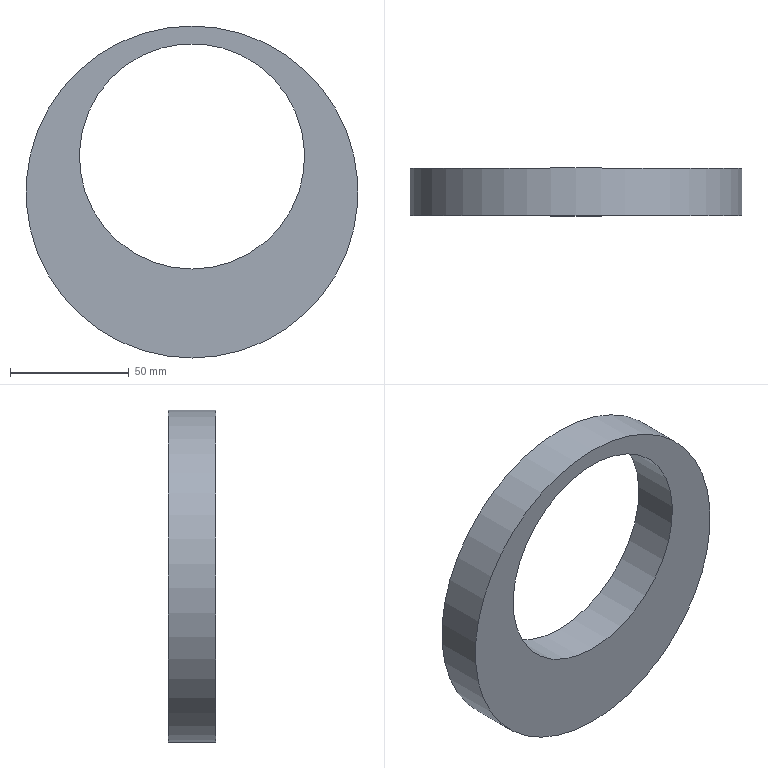Part | STEP file | 冲床-300配套压波_id738_x_t | 1 solid | 4 faces | box 140 x 20 x 140 mm | volume 166112 mm3 | plane 2 | cylinder 2 | commonest cylinder face diameters 95 x1 140 x1
STEP:
#1=CARTESIAN_POINT('',(2195.,-10.,-275.));
#2=VERTEX_POINT('',#1);
#3=CARTESIAN_POINT('',(2195.,-10.,-205.));
#4=DIRECTION('',(0.,1.,0.));
#5=DIRECTION('',(0.,0.,-1.));
#6=AXIS2_PLACEMENT_3D('',#3,#4,#5);
#7=CIRCLE('',#6,70.);
#8=EDGE_CURVE('',#2,#2,#7,.T.);
#9=ORIENTED_EDGE('',*,*,#8,.F.);
#10=EDGE_LOOP('',(#9));
#11=FACE_BOUND('',#10,.T.);
#12=CARTESIAN_POINT('',(2195.,-10.,-237.5));
#13=VERTEX_POINT('',#12);
#14=CARTESIAN_POINT('',(2195.,-10.,-190.));
#15=DIRECTION('',(0.,1.,0.));
#16=DIRECTION('',(0.,0.,-1.));
#17=AXIS2_PLACEMENT_3D('',#14,#15,#16);
#18=CIRCLE('',#17,47.5);
#19=EDGE_CURVE('',#13,#13,#18,.T.);
#20=ORIENTED_EDGE('',*,*,#19,.T.);
#21=EDGE_LOOP('',(#20));
#22=FACE_BOUND('',#21,.T.);
#23=CARTESIAN_POINT('',(432.953,-10.,916.258));
#24=DIRECTION('',(0.,-1.,0.));
#25=DIRECTION('',(-0.5361,0.,-0.8442));
#26=AXIS2_PLACEMENT_3D('',#23,#24,#25);
#27=PLANE('',#26);
#28=ADVANCED_FACE('',(#11,#22),#27,.T.);
#29=CARTESIAN_POINT('',(2195.,10.,-275.));
#30=VERTEX_POINT('',#29);
#31=CARTESIAN_POINT('',(2195.,10.,-205.));
#32=DIRECTION('',(0.,1.,0.));
#33=DIRECTION('',(0.,0.,-1.));
#34=AXIS2_PLACEMENT_3D('',#31,#32,#33);
#35=CIRCLE('',#34,70.);
#36=EDGE_CURVE('',#30,#30,#35,.T.);
#37=ORIENTED_EDGE('',*,*,#36,.T.);
#38=EDGE_LOOP('',(#37));
#39=FACE_BOUND('',#38,.T.);
#40=CARTESIAN_POINT('',(2195.,10.,-237.5));
#41=VERTEX_POINT('',#40);
#42=CARTESIAN_POINT('',(2195.,10.,-190.));
#43=DIRECTION('',(0.,1.,0.));
#44=DIRECTION('',(0.,0.,-1.));
#45=AXIS2_PLACEMENT_3D('',#42,#43,#44);
#46=CIRCLE('',#45,47.5);
#47=EDGE_CURVE('',#41,#41,#46,.T.);
#48=ORIENTED_EDGE('',*,*,#47,.F.);
#49=EDGE_LOOP('',(#48));
#50=FACE_BOUND('',#49,.T.);
#51=CARTESIAN_POINT('',(432.953,10.,916.258));
#52=DIRECTION('',(0.,-1.,0.));
#53=DIRECTION('',(-0.5361,0.,-0.8442));
#54=AXIS2_PLACEMENT_3D('',#51,#52,#53);
#55=PLANE('',#54);
#56=ADVANCED_FACE('',(#39,#50),#55,.F.);
#57=ORIENTED_EDGE('',*,*,#8,.T.);
#58=EDGE_LOOP('',(#57));
#59=FACE_BOUND('',#58,.T.);
#60=ORIENTED_EDGE('',*,*,#36,.F.);
#61=EDGE_LOOP('',(#60));
#62=FACE_BOUND('',#61,.T.);
#63=CARTESIAN_POINT('',(2195.,-71.,-205.));
#64=DIRECTION('',(0.,1.,0.));
#65=DIRECTION('',(0.,0.,1.));
#66=AXIS2_PLACEMENT_3D('',#63,#64,#65);
#67=CYLINDRICAL_SURFACE('',#66,70.);
#68=ADVANCED_FACE('',(#59,#62),#67,.T.);
#69=ORIENTED_EDGE('',*,*,#19,.F.);
#70=EDGE_LOOP('',(#69));
#71=FACE_BOUND('',#70,.T.);
#72=ORIENTED_EDGE('',*,*,#47,.T.);
#73=EDGE_LOOP('',(#72));
#74=FACE_BOUND('',#73,.T.);
#75=CARTESIAN_POINT('',(2195.,-26.5,-190.));
#76=DIRECTION('',(0.,1.,0.));
#77=DIRECTION('',(-0.7071,0.,0.7071));
#78=AXIS2_PLACEMENT_3D('',#75,#76,#77);
#79=CYLINDRICAL_SURFACE('',#78,47.5);
#80=ADVANCED_FACE('',(#71,#74),#79,.F.);
#81=CLOSED_SHELL('',(#28,#56,#68,#80));
#82=MANIFOLD_SOLID_BREP('',#81);
#83=(LENGTH_UNIT()NAMED_UNIT(*)SI_UNIT(.MILLI.,.METRE.));
#84=UNCERTAINTY_MEASURE_WITH_UNIT(LENGTH_MEASURE(0.00002),#83,'','');
#85=(NAMED_UNIT(*)PLANE_ANGLE_UNIT()SI_UNIT($,.RADIAN.));
#86=PLANE_ANGLE_MEASURE_WITH_UNIT(PLANE_ANGLE_MEASURE(0.01745),#85);
#87=DIMENSIONAL_EXPONENTS(0.,0.,0.,0.,0.,0.,0.);
#88=(CONVERSION_BASED_UNIT('DEGREE',#86)NAMED_UNIT(#87)PLANE_ANGLE_UNIT());
#89=(NAMED_UNIT(*)SI_UNIT($,.STERADIAN.)SOLID_ANGLE_UNIT());
#90=(GEOMETRIC_REPRESENTATION_CONTEXT(3)GLOBAL_UNCERTAINTY_ASSIGNED_CONTEXT((#84))GLOBAL_UNIT_ASSIGNED_CONTEXT((#83,#88,#89))REPRESENTATION_CONTEXT('',''));
#91=ADVANCED_BREP_SHAPE_REPRESENTATION('',(#82),#90);